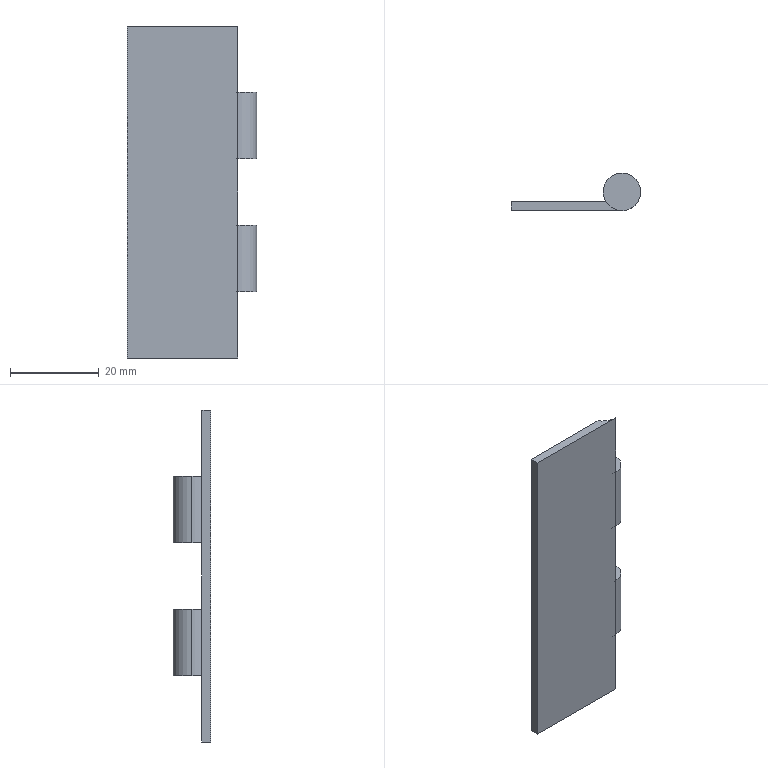Part | STEP file | _PDHFA2-75.step | 1 solid | 18 faces | box 29.25 x 8.5 x 75 mm | volume 5070 mm3 | cylinder 9 | plane 9 | commonest cylinder face diameters 8.5 x9
STEP:
#1=CARTESIAN_POINT('',(0.,0.,0.));
#2=DIRECTION('',(0.,0.,1.));
#3=DIRECTION('',(1.,0.,0.));
#4=AXIS2_PLACEMENT_3D('',#1,#2,#3);
#5=CARTESIAN_POINT('',(0.,0.,15.));
#6=VERTEX_POINT('',#5);
#7=CARTESIAN_POINT('',(4.25,4.25,15.));
#8=VERTEX_POINT('',#7);
#9=CARTESIAN_POINT('',(0.,4.25,15.));
#10=DIRECTION('',(0.,0.,1.));
#11=DIRECTION('',(1.,0.,0.));
#12=AXIS2_PLACEMENT_3D('',#9,#10,#11);
#13=CIRCLE('',#12,4.25);
#14=CARTESIAN_POINT('',(0.,4.25,75.));
#15=DIRECTION('',(0.,0.,1.));
#16=DIRECTION('',(-1.,0.,0.));
#17=AXIS2_PLACEMENT_3D('',#14,#15,#16);
#18=CYLINDRICAL_SURFACE('',#17,4.25);
#19=CARTESIAN_POINT('',(-3.142,-60.));
#20=DIRECTION('',(1.,0.));
#21=VECTOR('',#20,1.);
#22=LINE('',#19,#21);
#23=(GEOMETRIC_REPRESENTATION_CONTEXT(2)PARAMETRIC_REPRESENTATION_CONTEXT()REPRESENTATION_CONTEXT('',''));
#24=DEFINITIONAL_REPRESENTATION('',(#22),#23);
#25=PCURVE('',#18,#24);
#26=CARTESIAN_POINT('',(0.,4.25,15.));
#27=DIRECTION('',(0.,0.,1.));
#28=DIRECTION('',(1.,0.,0.));
#29=AXIS2_PLACEMENT_3D('',#26,#27,#28);
#30=PLANE('',#29);
#31=CARTESIAN_POINT('',(0.,0.));
#32=DIRECTION('',(1.,0.));
#33=AXIS2_PLACEMENT_2D('',#31,#32);
#34=CIRCLE('',#33,4.25);
#35=(GEOMETRIC_REPRESENTATION_CONTEXT(2)PARAMETRIC_REPRESENTATION_CONTEXT()REPRESENTATION_CONTEXT('',''));
#36=DEFINITIONAL_REPRESENTATION('',(#34),#35);
#37=PCURVE('',#30,#36);
#38=SURFACE_CURVE('',#13,(#25,#37),.PCURVE_S1.);
#39=EDGE_CURVE('',#6,#8,#38,.T.);
#40=ORIENTED_EDGE('',*,*,#39,.T.);
#41=CARTESIAN_POINT('',(4.25,4.25,30.));
#42=VERTEX_POINT('',#41);
#43=CARTESIAN_POINT('',(4.25,4.25,75.));
#44=DIRECTION('',(0.,0.,1.));
#45=VECTOR('',#44,1.);
#46=LINE('',#43,#45);
#47=CARTESIAN_POINT('',(3.142,0.));
#48=DIRECTION('',(0.,1.));
#49=VECTOR('',#48,1.);
#50=LINE('',#47,#49);
#51=(GEOMETRIC_REPRESENTATION_CONTEXT(2)PARAMETRIC_REPRESENTATION_CONTEXT()REPRESENTATION_CONTEXT('',''));
#52=DEFINITIONAL_REPRESENTATION('',(#50),#51);
#53=PCURVE('',#18,#52);
#54=CARTESIAN_POINT('',(0.,4.25,75.));
#55=DIRECTION('',(0.,0.,1.));
#56=DIRECTION('',(-1.,0.,0.));
#57=AXIS2_PLACEMENT_3D('',#54,#55,#56);
#58=CYLINDRICAL_SURFACE('',#57,4.25);
#59=CARTESIAN_POINT('',(3.142,0.));
#60=DIRECTION('',(0.,1.));
#61=VECTOR('',#60,1.);
#62=LINE('',#59,#61);
#63=(GEOMETRIC_REPRESENTATION_CONTEXT(2)PARAMETRIC_REPRESENTATION_CONTEXT()REPRESENTATION_CONTEXT('',''));
#64=DEFINITIONAL_REPRESENTATION('',(#62),#63);
#65=PCURVE('',#58,#64);
#66=SURFACE_CURVE('',#46,(#53,#65),.PCURVE_S1.);
#67=EDGE_CURVE('',#8,#42,#66,.T.);
#68=ORIENTED_EDGE('',*,*,#67,.T.);
#69=CARTESIAN_POINT('',(0.,0.,30.));
#70=VERTEX_POINT('',#69);
#71=CARTESIAN_POINT('',(0.,4.25,30.));
#72=DIRECTION('',(0.,0.,1.));
#73=DIRECTION('',(1.,0.,0.));
#74=AXIS2_PLACEMENT_3D('',#71,#72,#73);
#75=CIRCLE('',#74,4.25);
#76=CARTESIAN_POINT('',(-3.142,-45.));
#77=DIRECTION('',(1.,0.));
#78=VECTOR('',#77,1.);
#79=LINE('',#76,#78);
#80=(GEOMETRIC_REPRESENTATION_CONTEXT(2)PARAMETRIC_REPRESENTATION_CONTEXT()REPRESENTATION_CONTEXT('',''));
#81=DEFINITIONAL_REPRESENTATION('',(#79),#80);
#82=PCURVE('',#18,#81);
#83=CARTESIAN_POINT('',(0.,4.25,30.));
#84=DIRECTION('',(0.,0.,1.));
#85=DIRECTION('',(1.,0.,0.));
#86=AXIS2_PLACEMENT_3D('',#83,#84,#85);
#87=PLANE('',#86);
#88=CARTESIAN_POINT('',(0.,0.));
#89=DIRECTION('',(1.,0.));
#90=AXIS2_PLACEMENT_2D('',#88,#89);
#91=CIRCLE('',#90,4.25);
#92=(GEOMETRIC_REPRESENTATION_CONTEXT(2)PARAMETRIC_REPRESENTATION_CONTEXT()REPRESENTATION_CONTEXT('',''));
#93=DEFINITIONAL_REPRESENTATION('',(#91),#92);
#94=PCURVE('',#87,#93);
#95=SURFACE_CURVE('',#75,(#82,#94),.PCURVE_S1.);
#96=EDGE_CURVE('',#70,#42,#95,.T.);
#97=ORIENTED_EDGE('',*,*,#96,.F.);
#98=CARTESIAN_POINT('',(0.,0.,75.));
#99=DIRECTION('',(0.,0.,-1.));
#100=VECTOR('',#99,1.);
#101=LINE('',#98,#100);
#102=CARTESIAN_POINT('',(1.571,0.));
#103=DIRECTION('',(0.,-1.));
#104=VECTOR('',#103,1.);
#105=LINE('',#102,#104);
#106=(GEOMETRIC_REPRESENTATION_CONTEXT(2)PARAMETRIC_REPRESENTATION_CONTEXT()REPRESENTATION_CONTEXT('',''));
#107=DEFINITIONAL_REPRESENTATION('',(#105),#106);
#108=PCURVE('',#18,#107);
#109=CARTESIAN_POINT('',(-25.,0.,75.));
#110=DIRECTION('',(0.,1.,0.));
#111=DIRECTION('',(1.,0.,0.));
#112=AXIS2_PLACEMENT_3D('',#109,#110,#111);
#113=PLANE('',#112);
#114=CARTESIAN_POINT('',(25.,0.));
#115=DIRECTION('',(0.,1.));
#116=VECTOR('',#115,1.);
#117=LINE('',#114,#116);
#118=(GEOMETRIC_REPRESENTATION_CONTEXT(2)PARAMETRIC_REPRESENTATION_CONTEXT()REPRESENTATION_CONTEXT('',''));
#119=DEFINITIONAL_REPRESENTATION('',(#117),#118);
#120=PCURVE('',#113,#119);
#121=SURFACE_CURVE('',#101,(#108,#120),.PCURVE_S1.);
#122=EDGE_CURVE('',#70,#6,#121,.T.);
#123=ORIENTED_EDGE('',*,*,#122,.T.);
#124=EDGE_LOOP('',(#40,#68,#97,#123));
#125=FACE_BOUND('',#124,.T.);
#126=ADVANCED_FACE('',(#125),#18,.T.);
#127=ORIENTED_EDGE('',*,*,#67,.F.);
#128=CARTESIAN_POINT('',(-4.25,4.25,15.));
#129=VERTEX_POINT('',#128);
#130=CARTESIAN_POINT('',(0.,4.25,15.));
#131=DIRECTION('',(0.,0.,1.));
#132=DIRECTION('',(1.,0.,0.));
#133=AXIS2_PLACEMENT_3D('',#130,#131,#132);
#134=CIRCLE('',#133,4.25);
#135=CARTESIAN_POINT('',(3.142,-60.));
#136=DIRECTION('',(1.,0.));
#137=VECTOR('',#136,1.);
#138=LINE('',#135,#137);
#139=(GEOMETRIC_REPRESENTATION_CONTEXT(2)PARAMETRIC_REPRESENTATION_CONTEXT()REPRESENTATION_CONTEXT('',''));
#140=DEFINITIONAL_REPRESENTATION('',(#138),#139);
#141=PCURVE('',#58,#140);
#142=CARTESIAN_POINT('',(0.,0.));
#143=DIRECTION('',(1.,0.));
#144=AXIS2_PLACEMENT_2D('',#142,#143);
#145=CIRCLE('',#144,4.25);
#146=(GEOMETRIC_REPRESENTATION_CONTEXT(2)PARAMETRIC_REPRESENTATION_CONTEXT()REPRESENTATION_CONTEXT('',''));
#147=DEFINITIONAL_REPRESENTATION('',(#145),#146);
#148=PCURVE('',#30,#147);
#149=SURFACE_CURVE('',#134,(#141,#148),.PCURVE_S1.);
#150=EDGE_CURVE('',#8,#129,#149,.T.);
#151=ORIENTED_EDGE('',*,*,#150,.T.);
#152=CARTESIAN_POINT('',(-4.25,4.25,30.));
#153=VERTEX_POINT('',#152);
#154=CARTESIAN_POINT('',(-4.25,4.25,75.));
#155=DIRECTION('',(0.,0.,1.));
#156=VECTOR('',#155,1.);
#157=LINE('',#154,#156);
#158=CARTESIAN_POINT('',(6.283,0.));
#159=DIRECTION('',(0.,1.));
#160=VECTOR('',#159,1.);
#161=LINE('',#158,#160);
#162=(GEOMETRIC_REPRESENTATION_CONTEXT(2)PARAMETRIC_REPRESENTATION_CONTEXT()REPRESENTATION_CONTEXT('',''));
#163=DEFINITIONAL_REPRESENTATION('',(#161),#162);
#164=PCURVE('',#58,#163);
#165=CARTESIAN_POINT('',(0.,4.25,75.));
#166=DIRECTION('',(0.,0.,1.));
#167=DIRECTION('',(-1.,0.,0.));
#168=AXIS2_PLACEMENT_3D('',#165,#166,#167);
#169=CYLINDRICAL_SURFACE('',#168,4.25);
#170=CARTESIAN_POINT('',(0.,0.));
#171=DIRECTION('',(0.,1.));
#172=VECTOR('',#171,1.);
#173=LINE('',#170,#172);
#174=(GEOMETRIC_REPRESENTATION_CONTEXT(2)PARAMETRIC_REPRESENTATION_CONTEXT()REPRESENTATION_CONTEXT('',''));
#175=DEFINITIONAL_REPRESENTATION('',(#173),#174);
#176=PCURVE('',#169,#175);
#177=SURFACE_CURVE('',#157,(#164,#176),.PCURVE_S1.);
#178=EDGE_CURVE('',#129,#153,#177,.T.);
#179=ORIENTED_EDGE('',*,*,#178,.T.);
#180=CARTESIAN_POINT('',(0.,4.25,30.));
#181=DIRECTION('',(0.,0.,1.));
#182=DIRECTION('',(1.,0.,0.));
#183=AXIS2_PLACEMENT_3D('',#180,#181,#182);
#184=CIRCLE('',#183,4.25);
#185=CARTESIAN_POINT('',(3.142,-45.));
#186=DIRECTION('',(1.,0.));
#187=VECTOR('',#186,1.);
#188=LINE('',#185,#187);
#189=(GEOMETRIC_REPRESENTATION_CONTEXT(2)PARAMETRIC_REPRESENTATION_CONTEXT()REPRESENTATION_CONTEXT('',''));
#190=DEFINITIONAL_REPRESENTATION('',(#188),#189);
#191=PCURVE('',#58,#190);
#192=CARTESIAN_POINT('',(0.,0.));
#193=DIRECTION('',(1.,0.));
#194=AXIS2_PLACEMENT_2D('',#192,#193);
#195=CIRCLE('',#194,4.25);
#196=(GEOMETRIC_REPRESENTATION_CONTEXT(2)PARAMETRIC_REPRESENTATION_CONTEXT()REPRESENTATION_CONTEXT('',''));
#197=DEFINITIONAL_REPRESENTATION('',(#195),#196);
#198=PCURVE('',#87,#197);
#199=SURFACE_CURVE('',#184,(#191,#198),.PCURVE_S1.);
#200=EDGE_CURVE('',#42,#153,#199,.T.);
#201=ORIENTED_EDGE('',*,*,#200,.F.);
#202=EDGE_LOOP('',(#127,#151,#179,#201));
#203=FACE_BOUND('',#202,.T.);
#204=ADVANCED_FACE('',(#203),#58,.T.);
#205=CARTESIAN_POINT('',(0.,0.,45.));
#206=VERTEX_POINT('',#205);
#207=CARTESIAN_POINT('',(4.25,4.25,45.));
#208=VERTEX_POINT('',#207);
#209=CARTESIAN_POINT('',(0.,4.25,45.));
#210=DIRECTION('',(0.,0.,1.));
#211=DIRECTION('',(1.,0.,0.));
#212=AXIS2_PLACEMENT_3D('',#209,#210,#211);
#213=CIRCLE('',#212,4.25);
#214=CARTESIAN_POINT('',(0.,4.25,75.));
#215=DIRECTION('',(0.,0.,1.));
#216=DIRECTION('',(-1.,0.,0.));
#217=AXIS2_PLACEMENT_3D('',#214,#215,#216);
#218=CYLINDRICAL_SURFACE('',#217,4.25);
#219=CARTESIAN_POINT('',(-3.142,-30.));
#220=DIRECTION('',(1.,0.));
#221=VECTOR('',#220,1.);
#222=LINE('',#219,#221);
#223=(GEOMETRIC_REPRESENTATION_CONTEXT(2)PARAMETRIC_REPRESENTATION_CONTEXT()REPRESENTATION_CONTEXT('',''));
#224=DEFINITIONAL_REPRESENTATION('',(#222),#223);
#225=PCURVE('',#218,#224);
#226=CARTESIAN_POINT('',(0.,4.25,45.));
#227=DIRECTION('',(0.,0.,1.));
#228=DIRECTION('',(1.,0.,0.));
#229=AXIS2_PLACEMENT_3D('',#226,#227,#228);
#230=PLANE('',#229);
#231=CARTESIAN_POINT('',(0.,0.));
#232=DIRECTION('',(1.,0.));
#233=AXIS2_PLACEMENT_2D('',#231,#232);
#234=CIRCLE('',#233,4.25);
#235=(GEOMETRIC_REPRESENTATION_CONTEXT(2)PARAMETRIC_REPRESENTATION_CONTEXT()REPRESENTATION_CONTEXT('',''));
#236=DEFINITIONAL_REPRESENTATION('',(#234),#235);
#237=PCURVE('',#230,#236);
#238=SURFACE_CURVE('',#213,(#225,#237),.PCURVE_S1.);
#239=EDGE_CURVE('',#206,#208,#238,.T.);
#240=ORIENTED_EDGE('',*,*,#239,.T.);
#241=CARTESIAN_POINT('',(4.25,4.25,60.));
#242=VERTEX_POINT('',#241);
#243=CARTESIAN_POINT('',(4.25,4.25,75.));
#244=DIRECTION('',(0.,0.,1.));
#245=VECTOR('',#244,1.);
#246=LINE('',#243,#245);
#247=CARTESIAN_POINT('',(3.142,0.));
#248=DIRECTION('',(0.,1.));
#249=VECTOR('',#248,1.);
#250=LINE('',#247,#249);
#251=(GEOMETRIC_REPRESENTATION_CONTEXT(2)PARAMETRIC_REPRESENTATION_CONTEXT()REPRESENTATION_CONTEXT('',''));
#252=DEFINITIONAL_REPRESENTATION('',(#250),#251);
#253=PCURVE('',#218,#252);
#254=CARTESIAN_POINT('',(0.,4.25,75.));
#255=DIRECTION('',(0.,0.,1.));
#256=DIRECTION('',(-1.,0.,0.));
#257=AXIS2_PLACEMENT_3D('',#254,#255,#256);
#258=CYLINDRICAL_SURFACE('',#257,4.25);
#259=CARTESIAN_POINT('',(3.142,0.));
#260=DIRECTION('',(0.,1.));
#261=VECTOR('',#260,1.);
#262=LINE('',#259,#261);
#263=(GEOMETRIC_REPRESENTATION_CONTEXT(2)PARAMETRIC_REPRESENTATION_CONTEXT()REPRESENTATION_CONTEXT('',''));
#264=DEFINITIONAL_REPRESENTATION('',(#262),#263);
#265=PCURVE('',#258,#264);
#266=SURFACE_CURVE('',#246,(#253,#265),.PCURVE_S1.);
#267=EDGE_CURVE('',#208,#242,#266,.T.);
#268=ORIENTED_EDGE('',*,*,#267,.T.);
#269=CARTESIAN_POINT('',(0.,0.,60.));
#270=VERTEX_POINT('',#269);
#271=CARTESIAN_POINT('',(0.,4.25,60.));
#272=DIRECTION('',(0.,0.,1.));
#273=DIRECTION('',(1.,0.,0.));
#274=AXIS2_PLACEMENT_3D('',#271,#272,#273);
#275=CIRCLE('',#274,4.25);
#276=CARTESIAN_POINT('',(-3.142,-15.));
#277=DIRECTION('',(1.,0.));
#278=VECTOR('',#277,1.);
#279=LINE('',#276,#278);
#280=(GEOMETRIC_REPRESENTATION_CONTEXT(2)PARAMETRIC_REPRESENTATION_CONTEXT()REPRESENTATION_CONTEXT('',''));
#281=DEFINITIONAL_REPRESENTATION('',(#279),#280);
#282=PCURVE('',#218,#281);
#283=CARTESIAN_POINT('',(0.,4.25,60.));
#284=DIRECTION('',(0.,0.,1.));
#285=DIRECTION('',(1.,0.,0.));
#286=AXIS2_PLACEMENT_3D('',#283,#284,#285);
#287=PLANE('',#286);
#288=CARTESIAN_POINT('',(0.,0.));
#289=DIRECTION('',(1.,0.));
#290=AXIS2_PLACEMENT_2D('',#288,#289);
#291=CIRCLE('',#290,4.25);
#292=(GEOMETRIC_REPRESENTATION_CONTEXT(2)PARAMETRIC_REPRESENTATION_CONTEXT()REPRESENTATION_CONTEXT('',''));
#293=DEFINITIONAL_REPRESENTATION('',(#291),#292);
#294=PCURVE('',#287,#293);
#295=SURFACE_CURVE('',#275,(#282,#294),.PCURVE_S1.);
#296=EDGE_CURVE('',#270,#242,#295,.T.);
#297=ORIENTED_EDGE('',*,*,#296,.F.);
#298=CARTESIAN_POINT('',(0.,0.,75.));
#299=DIRECTION('',(0.,0.,-1.));
#300=VECTOR('',#299,1.);
#301=LINE('',#298,#300);
#302=CARTESIAN_POINT('',(1.571,0.));
#303=DIRECTION('',(0.,-1.));
#304=VECTOR('',#303,1.);
#305=LINE('',#302,#304);
#306=(GEOMETRIC_REPRESENTATION_CONTEXT(2)PARAMETRIC_REPRESENTATION_CONTEXT()REPRESENTATION_CONTEXT('',''));
#307=DEFINITIONAL_REPRESENTATION('',(#305),#306);
#308=PCURVE('',#218,#307);
#309=CARTESIAN_POINT('',(25.,0.));
#310=DIRECTION('',(0.,1.));
#311=VECTOR('',#310,1.);
#312=LINE('',#309,#311);
#313=(GEOMETRIC_REPRESENTATION_CONTEXT(2)PARAMETRIC_REPRESENTATION_CONTEXT()REPRESENTATION_CONTEXT('',''));
#314=DEFINITIONAL_REPRESENTATION('',(#312),#313);
#315=PCURVE('',#113,#314);
#316=SURFACE_CURVE('',#301,(#308,#315),.PCURVE_S1.);
#317=EDGE_CURVE('',#270,#206,#316,.T.);
#318=ORIENTED_EDGE('',*,*,#317,.T.);
#319=EDGE_LOOP('',(#240,#268,#297,#318));
#320=FACE_BOUND('',#319,.T.);
#321=ADVANCED_FACE('',(#320),#218,.T.);
#322=ORIENTED_EDGE('',*,*,#267,.F.);
#323=CARTESIAN_POINT('',(-4.25,4.25,45.));
#324=VERTEX_POINT('',#323);
#325=CARTESIAN_POINT('',(0.,4.25,45.));
#326=DIRECTION('',(0.,0.,1.));
#327=DIRECTION('',(1.,0.,0.));
#328=AXIS2_PLACEMENT_3D('',#325,#326,#327);
#329=CIRCLE('',#328,4.25);
#330=CARTESIAN_POINT('',(3.142,-30.));
#331=DIRECTION('',(1.,0.));
#332=VECTOR('',#331,1.);
#333=LINE('',#330,#332);
#334=(GEOMETRIC_REPRESENTATION_CONTEXT(2)PARAMETRIC_REPRESENTATION_CONTEXT()REPRESENTATION_CONTEXT('',''));
#335=DEFINITIONAL_REPRESENTATION('',(#333),#334);
#336=PCURVE('',#258,#335);
#337=CARTESIAN_POINT('',(0.,0.));
#338=DIRECTION('',(1.,0.));
#339=AXIS2_PLACEMENT_2D('',#337,#338);
#340=CIRCLE('',#339,4.25);
#341=(GEOMETRIC_REPRESENTATION_CONTEXT(2)PARAMETRIC_REPRESENTATION_CONTEXT()REPRESENTATION_CONTEXT('',''));
#342=DEFINITIONAL_REPRESENTATION('',(#340),#341);
#343=PCURVE('',#230,#342);
#344=SURFACE_CURVE('',#329,(#336,#343),.PCURVE_S1.);
#345=EDGE_CURVE('',#208,#324,#344,.T.);
#346=ORIENTED_EDGE('',*,*,#345,.T.);
#347=CARTESIAN_POINT('',(-4.25,4.25,60.));
#348=VERTEX_POINT('',#347);
#349=CARTESIAN_POINT('',(-4.25,4.25,75.));
#350=DIRECTION('',(0.,0.,1.));
#351=VECTOR('',#350,1.);
#352=LINE('',#349,#351);
#353=CARTESIAN_POINT('',(6.283,0.));
#354=DIRECTION('',(0.,1.));
#355=VECTOR('',#354,1.);
#356=LINE('',#353,#355);
#357=(GEOMETRIC_REPRESENTATION_CONTEXT(2)PARAMETRIC_REPRESENTATION_CONTEXT()REPRESENTATION_CONTEXT('',''));
#358=DEFINITIONAL_REPRESENTATION('',(#356),#357);
#359=PCURVE('',#258,#358);
#360=CARTESIAN_POINT('',(0.,4.25,75.));
#361=DIRECTION('',(0.,0.,1.));
#362=DIRECTION('',(-1.,0.,0.));
#363=AXIS2_PLACEMENT_3D('',#360,#361,#362);
#364=CYLINDRICAL_SURFACE('',#363,4.25);
#365=CARTESIAN_POINT('',(0.,0.));
#366=DIRECTION('',(0.,1.));
#367=VECTOR('',#366,1.);
#368=LINE('',#365,#367);
#369=(GEOMETRIC_REPRESENTATION_CONTEXT(2)PARAMETRIC_REPRESENTATION_CONTEXT()REPRESENTATION_CONTEXT('',''));
#370=DEFINITIONAL_REPRESENTATION('',(#368),#369);
#371=PCURVE('',#364,#370);
#372=SURFACE_CURVE('',#352,(#359,#371),.PCURVE_S1.);
#373=EDGE_CURVE('',#324,#348,#372,.T.);
#374=ORIENTED_EDGE('',*,*,#373,.T.);
#375=CARTESIAN_POINT('',(0.,4.25,60.));
#376=DIRECTION('',(0.,0.,1.));
#377=DIRECTION('',(1.,0.,0.));
#378=AXIS2_PLACEMENT_3D('',#375,#376,#377);
#379=CIRCLE('',#378,4.25);
#380=CARTESIAN_POINT('',(3.142,-15.));
#381=DIRECTION('',(1.,0.));
#382=VECTOR('',#381,1.);
#383=LINE('',#380,#382);
#384=(GEOMETRIC_REPRESENTATION_CONTEXT(2)PARAMETRIC_REPRESENTATION_CONTEXT()REPRESENTATION_CONTEXT('',''));
#385=DEFINITIONAL_REPRESENTATION('',(#383),#384);
#386=PCURVE('',#258,#385);
#387=CARTESIAN_POINT('',(0.,0.));
#388=DIRECTION('',(1.,0.));
#389=AXIS2_PLACEMENT_2D('',#387,#388);
#390=CIRCLE('',#389,4.25);
#391=(GEOMETRIC_REPRESENTATION_CONTEXT(2)PARAMETRIC_REPRESENTATION_CONTEXT()REPRESENTATION_CONTEXT('',''));
#392=DEFINITIONAL_REPRESENTATION('',(#390),#391);
#393=PCURVE('',#287,#392);
#394=SURFACE_CURVE('',#379,(#386,#393),.PCURVE_S1.);
#395=EDGE_CURVE('',#242,#348,#394,.T.);
#396=ORIENTED_EDGE('',*,*,#395,.F.);
#397=EDGE_LOOP('',(#322,#346,#374,#396));
#398=FACE_BOUND('',#397,.T.);
#399=ADVANCED_FACE('',(#398),#258,.T.);
#400=CARTESIAN_POINT('',(-3.606,2.,45.));
#401=VERTEX_POINT('',#400);
#402=CARTESIAN_POINT('',(0.,4.25,45.));
#403=DIRECTION('',(0.,0.,1.));
#404=DIRECTION('',(1.,0.,0.));
#405=AXIS2_PLACEMENT_3D('',#402,#403,#404);
#406=CIRCLE('',#405,4.25);
#407=CARTESIAN_POINT('',(0.,0.));
#408=DIRECTION('',(1.,0.));
#409=AXIS2_PLACEMENT_2D('',#407,#408);
#410=CIRCLE('',#409,4.25);
#411=(GEOMETRIC_REPRESENTATION_CONTEXT(2)PARAMETRIC_REPRESENTATION_CONTEXT()REPRESENTATION_CONTEXT('',''));
#412=DEFINITIONAL_REPRESENTATION('',(#410),#411);
#413=PCURVE('',#230,#412);
#414=CARTESIAN_POINT('',(0.,4.25,45.));
#415=DIRECTION('',(0.,0.,1.));
#416=DIRECTION('',(-1.,0.,0.));
#417=AXIS2_PLACEMENT_3D('',#414,#415,#416);
#418=CYLINDRICAL_SURFACE('',#417,4.25);
#419=CARTESIAN_POINT('',(-3.142,0.));
#420=DIRECTION('',(1.,0.));
#421=VECTOR('',#420,1.);
#422=LINE('',#419,#421);
#423=(GEOMETRIC_REPRESENTATION_CONTEXT(2)PARAMETRIC_REPRESENTATION_CONTEXT()REPRESENTATION_CONTEXT('',''));
#424=DEFINITIONAL_REPRESENTATION('',(#422),#423);
#425=PCURVE('',#418,#424);
#426=SURFACE_CURVE('',#406,(#413,#425),.PCURVE_S1.);
#427=EDGE_CURVE('',#401,#206,#426,.T.);
#428=ORIENTED_EDGE('',*,*,#427,.F.);
#429=CARTESIAN_POINT('',(0.,4.25,45.));
#430=DIRECTION('',(0.,0.,1.));
#431=DIRECTION('',(1.,0.,0.));
#432=AXIS2_PLACEMENT_3D('',#429,#430,#431);
#433=CIRCLE('',#432,4.25);
#434=CARTESIAN_POINT('',(0.,0.));
#435=DIRECTION('',(1.,0.));
#436=AXIS2_PLACEMENT_2D('',#434,#435);
#437=CIRCLE('',#436,4.25);
#438=(GEOMETRIC_REPRESENTATION_CONTEXT(2)PARAMETRIC_REPRESENTATION_CONTEXT()REPRESENTATION_CONTEXT('',''));
#439=DEFINITIONAL_REPRESENTATION('',(#437),#438);
#440=PCURVE('',#230,#439);
#441=CARTESIAN_POINT('',(-3.142,-30.));
#442=DIRECTION('',(1.,0.));
#443=VECTOR('',#442,1.);
#444=LINE('',#441,#443);
#445=(GEOMETRIC_REPRESENTATION_CONTEXT(2)PARAMETRIC_REPRESENTATION_CONTEXT()REPRESENTATION_CONTEXT('',''));
#446=DEFINITIONAL_REPRESENTATION('',(#444),#445);
#447=PCURVE('',#364,#446);
#448=SURFACE_CURVE('',#433,(#440,#447),.PCURVE_S1.);
#449=EDGE_CURVE('',#324,#401,#448,.T.);
#450=ORIENTED_EDGE('',*,*,#449,.F.);
#451=ORIENTED_EDGE('',*,*,#345,.F.);
#452=ORIENTED_EDGE('',*,*,#239,.F.);
#453=EDGE_LOOP('',(#428,#450,#451,#452));
#454=FACE_BOUND('',#453,.T.);
#455=ADVANCED_FACE('',(#454),#230,.F.);
#456=CARTESIAN_POINT('',(-3.606,2.,30.));
#457=VERTEX_POINT('',#456);
#458=CARTESIAN_POINT('',(0.,4.25,30.));
#459=DIRECTION('',(0.,0.,1.));
#460=DIRECTION('',(1.,0.,0.));
#461=AXIS2_PLACEMENT_3D('',#458,#459,#460);
#462=CIRCLE('',#461,4.25);
#463=CARTESIAN_POINT('',(0.,0.));
#464=DIRECTION('',(1.,0.));
#465=AXIS2_PLACEMENT_2D('',#463,#464);
#466=CIRCLE('',#465,4.25);
#467=(GEOMETRIC_REPRESENTATION_CONTEXT(2)PARAMETRIC_REPRESENTATION_CONTEXT()REPRESENTATION_CONTEXT('',''));
#468=DEFINITIONAL_REPRESENTATION('',(#466),#467);
#469=PCURVE('',#87,#468);
#470=CARTESIAN_POINT('',(-3.142,-15.));
#471=DIRECTION('',(1.,0.));
#472=VECTOR('',#471,1.);
#473=LINE('',#470,#472);
#474=(GEOMETRIC_REPRESENTATION_CONTEXT(2)PARAMETRIC_REPRESENTATION_CONTEXT()REPRESENTATION_CONTEXT('',''));
#475=DEFINITIONAL_REPRESENTATION('',(#473),#474);
#476=PCURVE('',#418,#475);
#477=SURFACE_CURVE('',#462,(#469,#476),.PCURVE_S1.);
#478=EDGE_CURVE('',#457,#70,#477,.T.);
#479=ORIENTED_EDGE('',*,*,#478,.T.);
#480=ORIENTED_EDGE('',*,*,#96,.T.);
#481=ORIENTED_EDGE('',*,*,#200,.T.);
#482=CARTESIAN_POINT('',(0.,4.25,30.));
#483=DIRECTION('',(0.,0.,1.));
#484=DIRECTION('',(1.,0.,0.));
#485=AXIS2_PLACEMENT_3D('',#482,#483,#484);
#486=CIRCLE('',#485,4.25);
#487=CARTESIAN_POINT('',(0.,0.));
#488=DIRECTION('',(1.,0.));
#489=AXIS2_PLACEMENT_2D('',#487,#488);
#490=CIRCLE('',#489,4.25);
#491=(GEOMETRIC_REPRESENTATION_CONTEXT(2)PARAMETRIC_REPRESENTATION_CONTEXT()REPRESENTATION_CONTEXT('',''));
#492=DEFINITIONAL_REPRESENTATION('',(#490),#491);
#493=PCURVE('',#87,#492);
#494=CARTESIAN_POINT('',(-3.142,-45.));
#495=DIRECTION('',(1.,0.));
#496=VECTOR('',#495,1.);
#497=LINE('',#494,#496);
#498=(GEOMETRIC_REPRESENTATION_CONTEXT(2)PARAMETRIC_REPRESENTATION_CONTEXT()REPRESENTATION_CONTEXT('',''));
#499=DEFINITIONAL_REPRESENTATION('',(#497),#498);
#500=PCURVE('',#169,#499);
#501=SURFACE_CURVE('',#486,(#493,#500),.PCURVE_S1.);
#502=EDGE_CURVE('',#153,#457,#501,.T.);
#503=ORIENTED_EDGE('',*,*,#502,.T.);
#504=EDGE_LOOP('',(#479,#480,#481,#503));
#505=FACE_BOUND('',#504,.T.);
#506=ADVANCED_FACE('',(#505),#87,.T.);
#507=ORIENTED_EDGE('',*,*,#478,.T.);
#508=CARTESIAN_POINT('',(0.,0.,75.));
#509=DIRECTION('',(0.,0.,-1.));
#510=VECTOR('',#509,1.);
#511=LINE('',#508,#510);
#512=CARTESIAN_POINT('',(1.571,30.));
#513=DIRECTION('',(0.,-1.));
#514=VECTOR('',#513,1.);
#515=LINE('',#512,#514);
#516=(GEOMETRIC_REPRESENTATION_CONTEXT(2)PARAMETRIC_REPRESENTATION_CONTEXT()REPRESENTATION_CONTEXT('',''));
#517=DEFINITIONAL_REPRESENTATION('',(#515),#516);
#518=PCURVE('',#418,#517);
#519=CARTESIAN_POINT('',(25.,0.));
#520=DIRECTION('',(0.,1.));
#521=VECTOR('',#520,1.);
#522=LINE('',#519,#521);
#523=(GEOMETRIC_REPRESENTATION_CONTEXT(2)PARAMETRIC_REPRESENTATION_CONTEXT()REPRESENTATION_CONTEXT('',''));
#524=DEFINITIONAL_REPRESENTATION('',(#522),#523);
#525=PCURVE('',#113,#524);
#526=SURFACE_CURVE('',#511,(#518,#525),.PCURVE_S1.);
#527=EDGE_CURVE('',#206,#70,#526,.T.);
#528=ORIENTED_EDGE('',*,*,#527,.F.);
#529=ORIENTED_EDGE('',*,*,#427,.F.);
#530=CARTESIAN_POINT('',(-3.606,2.,75.));
#531=DIRECTION('',(0.,0.,-1.));
#532=VECTOR('',#531,1.);
#533=LINE('',#530,#532);
#534=CARTESIAN_POINT('',(0.5579,30.));
#535=DIRECTION('',(0.,-1.));
#536=VECTOR('',#535,1.);
#537=LINE('',#534,#536);
#538=(GEOMETRIC_REPRESENTATION_CONTEXT(2)PARAMETRIC_REPRESENTATION_CONTEXT()REPRESENTATION_CONTEXT('',''));
#539=DEFINITIONAL_REPRESENTATION('',(#537),#538);
#540=PCURVE('',#418,#539);
#541=CARTESIAN_POINT('',(-3.606,2.,75.));
#542=DIRECTION('',(0.,-1.,0.));
#543=DIRECTION('',(0.,0.,-1.));
#544=AXIS2_PLACEMENT_3D('',#541,#542,#543);
#545=PLANE('',#544);
#546=CARTESIAN_POINT('',(0.,0.));
#547=DIRECTION('',(1.,0.));
#548=VECTOR('',#547,1.);
#549=LINE('',#546,#548);
#550=(GEOMETRIC_REPRESENTATION_CONTEXT(2)PARAMETRIC_REPRESENTATION_CONTEXT()REPRESENTATION_CONTEXT('',''));
#551=DEFINITIONAL_REPRESENTATION('',(#549),#550);
#552=PCURVE('',#545,#551);
#553=SURFACE_CURVE('',#533,(#540,#552),.PCURVE_S1.);
#554=EDGE_CURVE('',#401,#457,#553,.T.);
#555=ORIENTED_EDGE('',*,*,#554,.T.);
#556=EDGE_LOOP('',(#507,#528,#529,#555));
#557=FACE_BOUND('',#556,.F.);
#558=ADVANCED_FACE('',(#557),#418,.F.);
#559=ORIENTED_EDGE('',*,*,#373,.F.);
#560=ORIENTED_EDGE('',*,*,#449,.T.);
#561=CARTESIAN_POINT('',(-3.606,2.,60.));
#562=VERTEX_POINT('',#561);
#563=CARTESIAN_POINT('',(-3.606,2.,75.));
#564=DIRECTION('',(0.,0.,-1.));
#565=VECTOR('',#564,1.);
#566=LINE('',#563,#565);
#567=CARTESIAN_POINT('',(0.5579,0.));
#568=DIRECTION('',(0.,-1.));
#569=VECTOR('',#568,1.);
#570=LINE('',#567,#569);
#571=(GEOMETRIC_REPRESENTATION_CONTEXT(2)PARAMETRIC_REPRESENTATION_CONTEXT()REPRESENTATION_CONTEXT('',''));
#572=DEFINITIONAL_REPRESENTATION('',(#570),#571);
#573=PCURVE('',#364,#572);
#574=CARTESIAN_POINT('',(0.,0.));
#575=DIRECTION('',(1.,0.));
#576=VECTOR('',#575,1.);
#577=LINE('',#574,#576);
#578=(GEOMETRIC_REPRESENTATION_CONTEXT(2)PARAMETRIC_REPRESENTATION_CONTEXT()REPRESENTATION_CONTEXT('',''));
#579=DEFINITIONAL_REPRESENTATION('',(#577),#578);
#580=PCURVE('',#545,#579);
#581=SURFACE_CURVE('',#566,(#573,#580),.PCURVE_S1.);
#582=EDGE_CURVE('',#562,#401,#581,.T.);
#583=ORIENTED_EDGE('',*,*,#582,.F.);
#584=CARTESIAN_POINT('',(0.,4.25,60.));
#585=DIRECTION('',(0.,0.,1.));
#586=DIRECTION('',(1.,0.,0.));
#587=AXIS2_PLACEMENT_3D('',#584,#585,#586);
#588=CIRCLE('',#587,4.25);
#589=CARTESIAN_POINT('',(-3.142,-15.));
#590=DIRECTION('',(1.,0.));
#591=VECTOR('',#590,1.);
#592=LINE('',#589,#591);
#593=(GEOMETRIC_REPRESENTATION_CONTEXT(2)PARAMETRIC_REPRESENTATION_CONTEXT()REPRESENTATION_CONTEXT('',''));
#594=DEFINITIONAL_REPRESENTATION('',(#592),#593);
#595=PCURVE('',#364,#594);
#596=CARTESIAN_POINT('',(0.,0.));
#597=DIRECTION('',(1.,0.));
#598=AXIS2_PLACEMENT_2D('',#596,#597);
#599=CIRCLE('',#598,4.25);
#600=(GEOMETRIC_REPRESENTATION_CONTEXT(2)PARAMETRIC_REPRESENTATION_CONTEXT()REPRESENTATION_CONTEXT('',''));
#601=DEFINITIONAL_REPRESENTATION('',(#599),#600);
#602=PCURVE('',#287,#601);
#603=SURFACE_CURVE('',#588,(#595,#602),.PCURVE_S1.);
#604=EDGE_CURVE('',#348,#562,#603,.T.);
#605=ORIENTED_EDGE('',*,*,#604,.F.);
#606=EDGE_LOOP('',(#559,#560,#583,#605));
#607=FACE_BOUND('',#606,.T.);
#608=ADVANCED_FACE('',(#607),#364,.T.);
#609=CARTESIAN_POINT('',(-25.,0.,75.));
#610=VERTEX_POINT('',#609);
#611=CARTESIAN_POINT('',(0.,0.,75.));
#612=VERTEX_POINT('',#611);
#613=CARTESIAN_POINT('',(-25.,0.,75.));
#614=DIRECTION('',(1.,0.,0.));
#615=VECTOR('',#614,1.);
#616=LINE('',#613,#615);
#617=CARTESIAN_POINT('',(0.,4.25,75.));
#618=DIRECTION('',(0.,0.,1.));
#619=DIRECTION('',(1.,0.,0.));
#620=AXIS2_PLACEMENT_3D('',#617,#618,#619);
#621=PLANE('',#620);
#622=CARTESIAN_POINT('',(-25.,-4.25));
#623=DIRECTION('',(1.,0.));
#624=VECTOR('',#623,1.);
#625=LINE('',#622,#624);
#626=(GEOMETRIC_REPRESENTATION_CONTEXT(2)PARAMETRIC_REPRESENTATION_CONTEXT()REPRESENTATION_CONTEXT('',''));
#627=DEFINITIONAL_REPRESENTATION('',(#625),#626);
#628=PCURVE('',#621,#627);
#629=CARTESIAN_POINT('',(0.,0.));
#630=DIRECTION('',(1.,0.));
#631=VECTOR('',#630,1.);
#632=LINE('',#629,#631);
#633=(GEOMETRIC_REPRESENTATION_CONTEXT(2)PARAMETRIC_REPRESENTATION_CONTEXT()REPRESENTATION_CONTEXT('',''));
#634=DEFINITIONAL_REPRESENTATION('',(#632),#633);
#635=PCURVE('',#113,#634);
#636=SURFACE_CURVE('',#616,(#628,#635),.PCURVE_S1.);
#637=EDGE_CURVE('',#610,#612,#636,.T.);
#638=ORIENTED_EDGE('',*,*,#637,.T.);
#639=CARTESIAN_POINT('',(-3.606,2.,75.));
#640=VERTEX_POINT('',#639);
#641=CARTESIAN_POINT('',(0.,4.25,75.));
#642=DIRECTION('',(0.,0.,1.));
#643=DIRECTION('',(1.,0.,0.));
#644=AXIS2_PLACEMENT_3D('',#641,#642,#643);
#645=CIRCLE('',#644,4.25);
#646=CARTESIAN_POINT('',(0.,0.));
#647=DIRECTION('',(1.,0.));
#648=AXIS2_PLACEMENT_2D('',#646,#647);
#649=CIRCLE('',#648,4.25);
#650=(GEOMETRIC_REPRESENTATION_CONTEXT(2)PARAMETRIC_REPRESENTATION_CONTEXT()REPRESENTATION_CONTEXT('',''));
#651=DEFINITIONAL_REPRESENTATION('',(#649),#650);
#652=PCURVE('',#621,#651);
#653=CARTESIAN_POINT('',(0.,4.25,75.));
#654=DIRECTION('',(0.,0.,1.));
#655=DIRECTION('',(-1.,0.,0.));
#656=AXIS2_PLACEMENT_3D('',#653,#654,#655);
#657=CYLINDRICAL_SURFACE('',#656,4.25);
#658=CARTESIAN_POINT('',(-3.142,0.));
#659=DIRECTION('',(1.,0.));
#660=VECTOR('',#659,1.);
#661=LINE('',#658,#660);
#662=(GEOMETRIC_REPRESENTATION_CONTEXT(2)PARAMETRIC_REPRESENTATION_CONTEXT()REPRESENTATION_CONTEXT('',''));
#663=DEFINITIONAL_REPRESENTATION('',(#661),#662);
#664=PCURVE('',#657,#663);
#665=SURFACE_CURVE('',#645,(#652,#664),.PCURVE_S1.);
#666=EDGE_CURVE('',#640,#612,#665,.T.);
#667=ORIENTED_EDGE('',*,*,#666,.F.);
#668=CARTESIAN_POINT('',(-25.,2.,75.));
#669=VERTEX_POINT('',#668);
#670=CARTESIAN_POINT('',(-3.606,2.,75.));
#671=DIRECTION('',(-1.,0.,0.));
#672=VECTOR('',#671,1.);
#673=LINE('',#670,#672);
#674=CARTESIAN_POINT('',(-3.606,-2.25));
#675=DIRECTION('',(-1.,0.));
#676=VECTOR('',#675,1.);
#677=LINE('',#674,#676);
#678=(GEOMETRIC_REPRESENTATION_CONTEXT(2)PARAMETRIC_REPRESENTATION_CONTEXT()REPRESENTATION_CONTEXT('',''));
#679=DEFINITIONAL_REPRESENTATION('',(#677),#678);
#680=PCURVE('',#621,#679);
#681=CARTESIAN_POINT('',(0.,0.));
#682=DIRECTION('',(0.,-1.));
#683=VECTOR('',#682,1.);
#684=LINE('',#681,#683);
#685=(GEOMETRIC_REPRESENTATION_CONTEXT(2)PARAMETRIC_REPRESENTATION_CONTEXT()REPRESENTATION_CONTEXT('',''));
#686=DEFINITIONAL_REPRESENTATION('',(#684),#685);
#687=PCURVE('',#545,#686);
#688=SURFACE_CURVE('',#673,(#680,#687),.PCURVE_S1.);
#689=EDGE_CURVE('',#640,#669,#688,.T.);
#690=ORIENTED_EDGE('',*,*,#689,.T.);
#691=CARTESIAN_POINT('',(-25.,2.,75.));
#692=DIRECTION('',(0.,-1.,0.));
#693=VECTOR('',#692,1.);
#694=LINE('',#691,#693);
#695=CARTESIAN_POINT('',(-25.,-2.25));
#696=DIRECTION('',(0.,-1.));
#697=VECTOR('',#696,1.);
#698=LINE('',#695,#697);
#699=(GEOMETRIC_REPRESENTATION_CONTEXT(2)PARAMETRIC_REPRESENTATION_CONTEXT()REPRESENTATION_CONTEXT('',''));
#700=DEFINITIONAL_REPRESENTATION('',(#698),#699);
#701=PCURVE('',#621,#700);
#702=CARTESIAN_POINT('',(-25.,2.,75.));
#703=DIRECTION('',(1.,0.,0.));
#704=DIRECTION('',(0.,1.,0.));
#705=AXIS2_PLACEMENT_3D('',#702,#703,#704);
#706=PLANE('',#705);
#707=CARTESIAN_POINT('',(0.,0.));
#708=DIRECTION('',(-1.,0.));
#709=VECTOR('',#708,1.);
#710=LINE('',#707,#709);
#711=(GEOMETRIC_REPRESENTATION_CONTEXT(2)PARAMETRIC_REPRESENTATION_CONTEXT()REPRESENTATION_CONTEXT('',''));
#712=DEFINITIONAL_REPRESENTATION('',(#710),#711);
#713=PCURVE('',#706,#712);
#714=SURFACE_CURVE('',#694,(#701,#713),.PCURVE_S1.);
#715=EDGE_CURVE('',#669,#610,#714,.T.);
#716=ORIENTED_EDGE('',*,*,#715,.T.);
#717=EDGE_LOOP('',(#638,#667,#690,#716));
#718=FACE_BOUND('',#717,.T.);
#719=ADVANCED_FACE('',(#718),#621,.T.);
#720=ORIENTED_EDGE('',*,*,#178,.F.);
#721=CARTESIAN_POINT('',(-3.606,2.,15.));
#722=VERTEX_POINT('',#721);
#723=CARTESIAN_POINT('',(0.,4.25,15.));
#724=DIRECTION('',(0.,0.,1.));
#725=DIRECTION('',(1.,0.,0.));
#726=AXIS2_PLACEMENT_3D('',#723,#724,#725);
#727=CIRCLE('',#726,4.25);
#728=CARTESIAN_POINT('',(-3.142,-60.));
#729=DIRECTION('',(1.,0.));
#730=VECTOR('',#729,1.);
#731=LINE('',#728,#730);
#732=(GEOMETRIC_REPRESENTATION_CONTEXT(2)PARAMETRIC_REPRESENTATION_CONTEXT()REPRESENTATION_CONTEXT('',''));
#733=DEFINITIONAL_REPRESENTATION('',(#731),#732);
#734=PCURVE('',#169,#733);
#735=CARTESIAN_POINT('',(0.,0.));
#736=DIRECTION('',(1.,0.));
#737=AXIS2_PLACEMENT_2D('',#735,#736);
#738=CIRCLE('',#737,4.25);
#739=(GEOMETRIC_REPRESENTATION_CONTEXT(2)PARAMETRIC_REPRESENTATION_CONTEXT()REPRESENTATION_CONTEXT('',''));
#740=DEFINITIONAL_REPRESENTATION('',(#738),#739);
#741=PCURVE('',#30,#740);
#742=SURFACE_CURVE('',#727,(#734,#741),.PCURVE_S1.);
#743=EDGE_CURVE('',#129,#722,#742,.T.);
#744=ORIENTED_EDGE('',*,*,#743,.T.);
#745=CARTESIAN_POINT('',(-3.606,2.,75.));
#746=DIRECTION('',(0.,0.,-1.));
#747=VECTOR('',#746,1.);
#748=LINE('',#745,#747);
#749=CARTESIAN_POINT('',(0.5579,0.));
#750=DIRECTION('',(0.,-1.));
#751=VECTOR('',#750,1.);
#752=LINE('',#749,#751);
#753=(GEOMETRIC_REPRESENTATION_CONTEXT(2)PARAMETRIC_REPRESENTATION_CONTEXT()REPRESENTATION_CONTEXT('',''));
#754=DEFINITIONAL_REPRESENTATION('',(#752),#753);
#755=PCURVE('',#169,#754);
#756=CARTESIAN_POINT('',(0.,0.));
#757=DIRECTION('',(1.,0.));
#758=VECTOR('',#757,1.);
#759=LINE('',#756,#758);
#760=(GEOMETRIC_REPRESENTATION_CONTEXT(2)PARAMETRIC_REPRESENTATION_CONTEXT()REPRESENTATION_CONTEXT('',''));
#761=DEFINITIONAL_REPRESENTATION('',(#759),#760);
#762=PCURVE('',#545,#761);
#763=SURFACE_CURVE('',#748,(#755,#762),.PCURVE_S1.);
#764=EDGE_CURVE('',#457,#722,#763,.T.);
#765=ORIENTED_EDGE('',*,*,#764,.F.);
#766=ORIENTED_EDGE('',*,*,#502,.F.);
#767=EDGE_LOOP('',(#720,#744,#765,#766));
#768=FACE_BOUND('',#767,.T.);
#769=ADVANCED_FACE('',(#768),#169,.T.);
#770=CARTESIAN_POINT('',(-3.606,2.,0.));
#771=VERTEX_POINT('',#770);
#772=CARTESIAN_POINT('',(0.,0.,0.));
#773=VERTEX_POINT('',#772);
#774=CARTESIAN_POINT('',(0.,4.25,0.));
#775=DIRECTION('',(0.,0.,1.));
#776=DIRECTION('',(1.,0.,0.));
#777=AXIS2_PLACEMENT_3D('',#774,#775,#776);
#778=CIRCLE('',#777,4.25);
#779=CARTESIAN_POINT('',(0.,4.25,0.));
#780=DIRECTION('',(0.,0.,1.));
#781=DIRECTION('',(1.,0.,0.));
#782=AXIS2_PLACEMENT_3D('',#779,#780,#781);
#783=PLANE('',#782);
#784=CARTESIAN_POINT('',(0.,0.));
#785=DIRECTION('',(1.,0.));
#786=AXIS2_PLACEMENT_2D('',#784,#785);
#787=CIRCLE('',#786,4.25);
#788=(GEOMETRIC_REPRESENTATION_CONTEXT(2)PARAMETRIC_REPRESENTATION_CONTEXT()REPRESENTATION_CONTEXT('',''));
#789=DEFINITIONAL_REPRESENTATION('',(#787),#788);
#790=PCURVE('',#783,#789);
#791=CARTESIAN_POINT('',(0.,4.25,15.));
#792=DIRECTION('',(0.,0.,1.));
#793=DIRECTION('',(-1.,0.,0.));
#794=AXIS2_PLACEMENT_3D('',#791,#792,#793);
#795=CYLINDRICAL_SURFACE('',#794,4.25);
#796=CARTESIAN_POINT('',(-3.142,-15.));
#797=DIRECTION('',(1.,0.));
#798=VECTOR('',#797,1.);
#799=LINE('',#796,#798);
#800=(GEOMETRIC_REPRESENTATION_CONTEXT(2)PARAMETRIC_REPRESENTATION_CONTEXT()REPRESENTATION_CONTEXT('',''));
#801=DEFINITIONAL_REPRESENTATION('',(#799),#800);
#802=PCURVE('',#795,#801);
#803=SURFACE_CURVE('',#778,(#790,#802),.PCURVE_S1.);
#804=EDGE_CURVE('',#771,#773,#803,.T.);
#805=ORIENTED_EDGE('',*,*,#804,.T.);
#806=CARTESIAN_POINT('',(-25.,0.,0.));
#807=VERTEX_POINT('',#806);
#808=CARTESIAN_POINT('',(-25.,0.,0.));
#809=DIRECTION('',(1.,0.,0.));
#810=VECTOR('',#809,1.);
#811=LINE('',#808,#810);
#812=CARTESIAN_POINT('',(-25.,-4.25));
#813=DIRECTION('',(1.,0.));
#814=VECTOR('',#813,1.);
#815=LINE('',#812,#814);
#816=(GEOMETRIC_REPRESENTATION_CONTEXT(2)PARAMETRIC_REPRESENTATION_CONTEXT()REPRESENTATION_CONTEXT('',''));
#817=DEFINITIONAL_REPRESENTATION('',(#815),#816);
#818=PCURVE('',#783,#817);
#819=CARTESIAN_POINT('',(0.,75.));
#820=DIRECTION('',(1.,0.));
#821=VECTOR('',#820,1.);
#822=LINE('',#819,#821);
#823=(GEOMETRIC_REPRESENTATION_CONTEXT(2)PARAMETRIC_REPRESENTATION_CONTEXT()REPRESENTATION_CONTEXT('',''));
#824=DEFINITIONAL_REPRESENTATION('',(#822),#823);
#825=PCURVE('',#113,#824);
#826=SURFACE_CURVE('',#811,(#818,#825),.PCURVE_S1.);
#827=EDGE_CURVE('',#807,#773,#826,.T.);
#828=ORIENTED_EDGE('',*,*,#827,.F.);
#829=CARTESIAN_POINT('',(-25.,2.,0.));
#830=VERTEX_POINT('',#829);
#831=CARTESIAN_POINT('',(-25.,2.,0.));
#832=DIRECTION('',(0.,-1.,0.));
#833=VECTOR('',#832,1.);
#834=LINE('',#831,#833);
#835=CARTESIAN_POINT('',(-25.,-2.25));
#836=DIRECTION('',(0.,-1.));
#837=VECTOR('',#836,1.);
#838=LINE('',#835,#837);
#839=(GEOMETRIC_REPRESENTATION_CONTEXT(2)PARAMETRIC_REPRESENTATION_CONTEXT()REPRESENTATION_CONTEXT('',''));
#840=DEFINITIONAL_REPRESENTATION('',(#838),#839);
#841=PCURVE('',#783,#840);
#842=CARTESIAN_POINT('',(0.,-75.));
#843=DIRECTION('',(-1.,0.));
#844=VECTOR('',#843,1.);
#845=LINE('',#842,#844);
#846=(GEOMETRIC_REPRESENTATION_CONTEXT(2)PARAMETRIC_REPRESENTATION_CONTEXT()REPRESENTATION_CONTEXT('',''));
#847=DEFINITIONAL_REPRESENTATION('',(#845),#846);
#848=PCURVE('',#706,#847);
#849=SURFACE_CURVE('',#834,(#841,#848),.PCURVE_S1.);
#850=EDGE_CURVE('',#830,#807,#849,.T.);
#851=ORIENTED_EDGE('',*,*,#850,.F.);
#852=CARTESIAN_POINT('',(-3.606,2.,0.));
#853=DIRECTION('',(-1.,0.,0.));
#854=VECTOR('',#853,1.);
#855=LINE('',#852,#854);
#856=CARTESIAN_POINT('',(-3.606,-2.25));
#857=DIRECTION('',(-1.,0.));
#858=VECTOR('',#857,1.);
#859=LINE('',#856,#858);
#860=(GEOMETRIC_REPRESENTATION_CONTEXT(2)PARAMETRIC_REPRESENTATION_CONTEXT()REPRESENTATION_CONTEXT('',''));
#861=DEFINITIONAL_REPRESENTATION('',(#859),#860);
#862=PCURVE('',#783,#861);
#863=CARTESIAN_POINT('',(75.,0.));
#864=DIRECTION('',(0.,-1.));
#865=VECTOR('',#864,1.);
#866=LINE('',#863,#865);
#867=(GEOMETRIC_REPRESENTATION_CONTEXT(2)PARAMETRIC_REPRESENTATION_CONTEXT()REPRESENTATION_CONTEXT('',''));
#868=DEFINITIONAL_REPRESENTATION('',(#866),#867);
#869=PCURVE('',#545,#868);
#870=SURFACE_CURVE('',#855,(#862,#869),.PCURVE_S1.);
#871=EDGE_CURVE('',#771,#830,#870,.T.);
#872=ORIENTED_EDGE('',*,*,#871,.F.);
#873=EDGE_LOOP('',(#805,#828,#851,#872));
#874=FACE_BOUND('',#873,.T.);
#875=ADVANCED_FACE('',(#874),#783,.F.);
#876=ORIENTED_EDGE('',*,*,#871,.T.);
#877=CARTESIAN_POINT('',(-25.,2.,75.));
#878=DIRECTION('',(0.,0.,-1.));
#879=VECTOR('',#878,1.);
#880=LINE('',#877,#879);
#881=CARTESIAN_POINT('',(0.,-21.394));
#882=DIRECTION('',(1.,0.));
#883=VECTOR('',#882,1.);
#884=LINE('',#881,#883);
#885=(GEOMETRIC_REPRESENTATION_CONTEXT(2)PARAMETRIC_REPRESENTATION_CONTEXT()REPRESENTATION_CONTEXT('',''));
#886=DEFINITIONAL_REPRESENTATION('',(#884),#885);
#887=PCURVE('',#545,#886);
#888=CARTESIAN_POINT('',(0.,0.));
#889=DIRECTION('',(0.,-1.));
#890=VECTOR('',#889,1.);
#891=LINE('',#888,#890);
#892=(GEOMETRIC_REPRESENTATION_CONTEXT(2)PARAMETRIC_REPRESENTATION_CONTEXT()REPRESENTATION_CONTEXT('',''));
#893=DEFINITIONAL_REPRESENTATION('',(#891),#892);
#894=PCURVE('',#706,#893);
#895=SURFACE_CURVE('',#880,(#887,#894),.PCURVE_S1.);
#896=EDGE_CURVE('',#669,#830,#895,.T.);
#897=ORIENTED_EDGE('',*,*,#896,.F.);
#898=ORIENTED_EDGE('',*,*,#689,.F.);
#899=CARTESIAN_POINT('',(-3.606,2.,75.));
#900=DIRECTION('',(0.,0.,-1.));
#901=VECTOR('',#900,1.);
#902=LINE('',#899,#901);
#903=CARTESIAN_POINT('',(0.,0.));
#904=DIRECTION('',(1.,0.));
#905=VECTOR('',#904,1.);
#906=LINE('',#903,#905);
#907=(GEOMETRIC_REPRESENTATION_CONTEXT(2)PARAMETRIC_REPRESENTATION_CONTEXT()REPRESENTATION_CONTEXT('',''));
#908=DEFINITIONAL_REPRESENTATION('',(#906),#907);
#909=PCURVE('',#545,#908);
#910=CARTESIAN_POINT('',(0.5579,0.));
#911=DIRECTION('',(0.,-1.));
#912=VECTOR('',#911,1.);
#913=LINE('',#910,#912);
#914=(GEOMETRIC_REPRESENTATION_CONTEXT(2)PARAMETRIC_REPRESENTATION_CONTEXT()REPRESENTATION_CONTEXT('',''));
#915=DEFINITIONAL_REPRESENTATION('',(#913),#914);
#916=PCURVE('',#657,#915);
#917=SURFACE_CURVE('',#902,(#909,#916),.PCURVE_S1.);
#918=EDGE_CURVE('',#640,#562,#917,.T.);
#919=ORIENTED_EDGE('',*,*,#918,.T.);
#920=ORIENTED_EDGE('',*,*,#582,.T.);
#921=ORIENTED_EDGE('',*,*,#554,.T.);
#922=ORIENTED_EDGE('',*,*,#764,.T.);
#923=CARTESIAN_POINT('',(-3.606,2.,15.));
#924=DIRECTION('',(0.,0.,1.));
#925=VECTOR('',#924,1.);
#926=LINE('',#923,#925);
#927=CARTESIAN_POINT('',(60.,0.));
#928=DIRECTION('',(-1.,0.));
#929=VECTOR('',#928,1.);
#930=LINE('',#927,#929);
#931=(GEOMETRIC_REPRESENTATION_CONTEXT(2)PARAMETRIC_REPRESENTATION_CONTEXT()REPRESENTATION_CONTEXT('',''));
#932=DEFINITIONAL_REPRESENTATION('',(#930),#931);
#933=PCURVE('',#545,#932);
#934=CARTESIAN_POINT('',(0.5579,0.));
#935=DIRECTION('',(0.,1.));
#936=VECTOR('',#935,1.);
#937=LINE('',#934,#936);
#938=(GEOMETRIC_REPRESENTATION_CONTEXT(2)PARAMETRIC_REPRESENTATION_CONTEXT()REPRESENTATION_CONTEXT('',''));
#939=DEFINITIONAL_REPRESENTATION('',(#937),#938);
#940=PCURVE('',#795,#939);
#941=SURFACE_CURVE('',#926,(#933,#940),.PCURVE_S1.);
#942=EDGE_CURVE('',#771,#722,#941,.T.);
#943=ORIENTED_EDGE('',*,*,#942,.F.);
#944=EDGE_LOOP('',(#876,#897,#898,#919,#920,#921,#922,#943));
#945=FACE_BOUND('',#944,.T.);
#946=ADVANCED_FACE('',(#945),#545,.F.);
#947=ORIENTED_EDGE('',*,*,#804,.T.);
#948=CARTESIAN_POINT('',(0.,0.,15.));
#949=DIRECTION('',(0.,0.,1.));
#950=VECTOR('',#949,1.);
#951=LINE('',#948,#950);
#952=CARTESIAN_POINT('',(1.571,0.));
#953=DIRECTION('',(0.,1.));
#954=VECTOR('',#953,1.);
#955=LINE('',#952,#954);
#956=(GEOMETRIC_REPRESENTATION_CONTEXT(2)PARAMETRIC_REPRESENTATION_CONTEXT()REPRESENTATION_CONTEXT('',''));
#957=DEFINITIONAL_REPRESENTATION('',(#955),#956);
#958=PCURVE('',#795,#957);
#959=CARTESIAN_POINT('',(25.,60.));
#960=DIRECTION('',(0.,-1.));
#961=VECTOR('',#960,1.);
#962=LINE('',#959,#961);
#963=(GEOMETRIC_REPRESENTATION_CONTEXT(2)PARAMETRIC_REPRESENTATION_CONTEXT()REPRESENTATION_CONTEXT('',''));
#964=DEFINITIONAL_REPRESENTATION('',(#962),#963);
#965=PCURVE('',#113,#964);
#966=SURFACE_CURVE('',#951,(#958,#965),.PCURVE_S1.);
#967=EDGE_CURVE('',#773,#6,#966,.T.);
#968=ORIENTED_EDGE('',*,*,#967,.T.);
#969=CARTESIAN_POINT('',(0.,4.25,15.));
#970=DIRECTION('',(0.,0.,1.));
#971=DIRECTION('',(1.,0.,0.));
#972=AXIS2_PLACEMENT_3D('',#969,#970,#971);
#973=CIRCLE('',#972,4.25);
#974=CARTESIAN_POINT('',(-3.142,0.));
#975=DIRECTION('',(1.,0.));
#976=VECTOR('',#975,1.);
#977=LINE('',#974,#976);
#978=(GEOMETRIC_REPRESENTATION_CONTEXT(2)PARAMETRIC_REPRESENTATION_CONTEXT()REPRESENTATION_CONTEXT('',''));
#979=DEFINITIONAL_REPRESENTATION('',(#977),#978);
#980=PCURVE('',#795,#979);
#981=CARTESIAN_POINT('',(0.,0.));
#982=DIRECTION('',(1.,0.));
#983=AXIS2_PLACEMENT_2D('',#981,#982);
#984=CIRCLE('',#983,4.25);
#985=(GEOMETRIC_REPRESENTATION_CONTEXT(2)PARAMETRIC_REPRESENTATION_CONTEXT()REPRESENTATION_CONTEXT('',''));
#986=DEFINITIONAL_REPRESENTATION('',(#984),#985);
#987=PCURVE('',#30,#986);
#988=SURFACE_CURVE('',#973,(#980,#987),.PCURVE_S1.);
#989=EDGE_CURVE('',#722,#6,#988,.T.);
#990=ORIENTED_EDGE('',*,*,#989,.F.);
#991=ORIENTED_EDGE('',*,*,#942,.F.);
#992=EDGE_LOOP('',(#947,#968,#990,#991));
#993=FACE_BOUND('',#992,.F.);
#994=ADVANCED_FACE('',(#993),#795,.F.);
#995=ORIENTED_EDGE('',*,*,#989,.F.);
#996=ORIENTED_EDGE('',*,*,#743,.F.);
#997=ORIENTED_EDGE('',*,*,#150,.F.);
#998=ORIENTED_EDGE('',*,*,#39,.F.);
#999=EDGE_LOOP('',(#995,#996,#997,#998));
#1000=FACE_BOUND('',#999,.T.);
#1001=ADVANCED_FACE('',(#1000),#30,.F.);
#1002=ORIENTED_EDGE('',*,*,#827,.T.);
#1003=ORIENTED_EDGE('',*,*,#967,.T.);
#1004=ORIENTED_EDGE('',*,*,#122,.F.);
#1005=ORIENTED_EDGE('',*,*,#527,.F.);
#1006=ORIENTED_EDGE('',*,*,#317,.F.);
#1007=CARTESIAN_POINT('',(0.,0.,75.));
#1008=DIRECTION('',(0.,0.,-1.));
#1009=VECTOR('',#1008,1.);
#1010=LINE('',#1007,#1009);
#1011=CARTESIAN_POINT('',(25.,0.));
#1012=DIRECTION('',(0.,1.));
#1013=VECTOR('',#1012,1.);
#1014=LINE('',#1011,#1013);
#1015=(GEOMETRIC_REPRESENTATION_CONTEXT(2)PARAMETRIC_REPRESENTATION_CONTEXT()REPRESENTATION_CONTEXT('',''));
#1016=DEFINITIONAL_REPRESENTATION('',(#1014),#1015);
#1017=PCURVE('',#113,#1016);
#1018=CARTESIAN_POINT('',(1.571,0.));
#1019=DIRECTION('',(0.,-1.));
#1020=VECTOR('',#1019,1.);
#1021=LINE('',#1018,#1020);
#1022=(GEOMETRIC_REPRESENTATION_CONTEXT(2)PARAMETRIC_REPRESENTATION_CONTEXT()REPRESENTATION_CONTEXT('',''));
#1023=DEFINITIONAL_REPRESENTATION('',(#1021),#1022);
#1024=PCURVE('',#657,#1023);
#1025=SURFACE_CURVE('',#1010,(#1017,#1024),.PCURVE_S1.);
#1026=EDGE_CURVE('',#612,#270,#1025,.T.);
#1027=ORIENTED_EDGE('',*,*,#1026,.F.);
#1028=ORIENTED_EDGE('',*,*,#637,.F.);
#1029=CARTESIAN_POINT('',(-25.,0.,75.));
#1030=DIRECTION('',(0.,0.,-1.));
#1031=VECTOR('',#1030,1.);
#1032=LINE('',#1029,#1031);
#1033=CARTESIAN_POINT('',(0.,0.));
#1034=DIRECTION('',(0.,1.));
#1035=VECTOR('',#1034,1.);
#1036=LINE('',#1033,#1035);
#1037=(GEOMETRIC_REPRESENTATION_CONTEXT(2)PARAMETRIC_REPRESENTATION_CONTEXT()REPRESENTATION_CONTEXT('',''));
#1038=DEFINITIONAL_REPRESENTATION('',(#1036),#1037);
#1039=PCURVE('',#113,#1038);
#1040=CARTESIAN_POINT('',(-2.,0.));
#1041=DIRECTION('',(0.,-1.));
#1042=VECTOR('',#1041,1.);
#1043=LINE('',#1040,#1042);
#1044=(GEOMETRIC_REPRESENTATION_CONTEXT(2)PARAMETRIC_REPRESENTATION_CONTEXT()REPRESENTATION_CONTEXT('',''));
#1045=DEFINITIONAL_REPRESENTATION('',(#1043),#1044);
#1046=PCURVE('',#706,#1045);
#1047=SURFACE_CURVE('',#1032,(#1039,#1046),.PCURVE_S1.);
#1048=EDGE_CURVE('',#610,#807,#1047,.T.);
#1049=ORIENTED_EDGE('',*,*,#1048,.T.);
#1050=EDGE_LOOP('',(#1002,#1003,#1004,#1005,#1006,#1027,#1028,#1049));
#1051=FACE_BOUND('',#1050,.T.);
#1052=ADVANCED_FACE('',(#1051),#113,.F.);
#1053=ORIENTED_EDGE('',*,*,#850,.T.);
#1054=ORIENTED_EDGE('',*,*,#1048,.F.);
#1055=ORIENTED_EDGE('',*,*,#715,.F.);
#1056=ORIENTED_EDGE('',*,*,#896,.T.);
#1057=EDGE_LOOP('',(#1053,#1054,#1055,#1056));
#1058=FACE_BOUND('',#1057,.T.);
#1059=ADVANCED_FACE('',(#1058),#706,.F.);
#1060=CARTESIAN_POINT('',(0.,4.25,60.));
#1061=DIRECTION('',(0.,0.,1.));
#1062=DIRECTION('',(1.,0.,0.));
#1063=AXIS2_PLACEMENT_3D('',#1060,#1061,#1062);
#1064=CIRCLE('',#1063,4.25);
#1065=CARTESIAN_POINT('',(-3.142,-15.));
#1066=DIRECTION('',(1.,0.));
#1067=VECTOR('',#1066,1.);
#1068=LINE('',#1065,#1067);
#1069=(GEOMETRIC_REPRESENTATION_CONTEXT(2)PARAMETRIC_REPRESENTATION_CONTEXT()REPRESENTATION_CONTEXT('',''));
#1070=DEFINITIONAL_REPRESENTATION('',(#1068),#1069);
#1071=PCURVE('',#657,#1070);
#1072=CARTESIAN_POINT('',(0.,0.));
#1073=DIRECTION('',(1.,0.));
#1074=AXIS2_PLACEMENT_2D('',#1072,#1073);
#1075=CIRCLE('',#1074,4.25);
#1076=(GEOMETRIC_REPRESENTATION_CONTEXT(2)PARAMETRIC_REPRESENTATION_CONTEXT()REPRESENTATION_CONTEXT('',''));
#1077=DEFINITIONAL_REPRESENTATION('',(#1075),#1076);
#1078=PCURVE('',#287,#1077);
#1079=SURFACE_CURVE('',#1064,(#1071,#1078),.PCURVE_S1.);
#1080=EDGE_CURVE('',#562,#270,#1079,.T.);
#1081=ORIENTED_EDGE('',*,*,#1080,.T.);
#1082=ORIENTED_EDGE('',*,*,#1026,.F.);
#1083=ORIENTED_EDGE('',*,*,#666,.F.);
#1084=ORIENTED_EDGE('',*,*,#918,.T.);
#1085=EDGE_LOOP('',(#1081,#1082,#1083,#1084));
#1086=FACE_BOUND('',#1085,.F.);
#1087=ADVANCED_FACE('',(#1086),#657,.F.);
#1088=ORIENTED_EDGE('',*,*,#1080,.T.);
#1089=ORIENTED_EDGE('',*,*,#296,.T.);
#1090=ORIENTED_EDGE('',*,*,#395,.T.);
#1091=ORIENTED_EDGE('',*,*,#604,.T.);
#1092=EDGE_LOOP('',(#1088,#1089,#1090,#1091));
#1093=FACE_BOUND('',#1092,.T.);
#1094=ADVANCED_FACE('',(#1093),#287,.T.);
#1095=CLOSED_SHELL('',(#126,#204,#321,#399,#455,#506,#558,#608,#719,#769,#875,#946,#994,#1001,#1052,#1059,#1087,#1094));
#1096=MANIFOLD_SOLID_BREP('',#1095);
#1097=(LENGTH_UNIT()NAMED_UNIT(*)SI_UNIT(.MILLI.,.METRE.));
#1098=UNCERTAINTY_MEASURE_WITH_UNIT(LENGTH_MEASURE(0.0000001),#1097,'','');
#1099=(NAMED_UNIT(*)PLANE_ANGLE_UNIT()SI_UNIT($,.RADIAN.));
#1100=(NAMED_UNIT(*)SI_UNIT($,.STERADIAN.)SOLID_ANGLE_UNIT());
#1101=(GEOMETRIC_REPRESENTATION_CONTEXT(3)GLOBAL_UNCERTAINTY_ASSIGNED_CONTEXT((#1098))GLOBAL_UNIT_ASSIGNED_CONTEXT((#1097,#1099,#1100))REPRESENTATION_CONTEXT('',''));
#1102=ADVANCED_BREP_SHAPE_REPRESENTATION('',(#4,#1096),#1101);